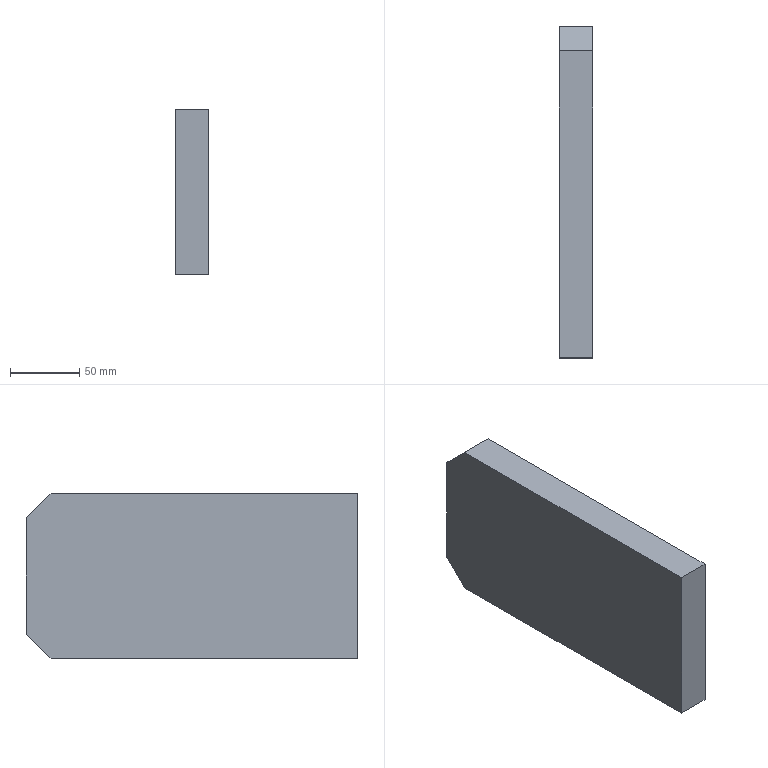Part | NX | 1 solid | 8 faces | box 24 x 240 x 120 mm | volume 683424 mm3 | plane 8
STEP:
#1=CARTESIAN_POINT('',(-235.326,-487.347,2383.086));
#2=VERTEX_POINT('',#1);
#3=CARTESIAN_POINT('',(-235.326,-487.347,2467.086));
#4=VERTEX_POINT('',#3);
#5=CARTESIAN_POINT('',(-235.326,-487.347,2485.086));
#6=DIRECTION('',(0.,0.,1.));
#7=VECTOR('',#6,1.);
#8=LINE('',#5,#7);
#9=EDGE_CURVE('',#2,#4,#8,.T.);
#10=ORIENTED_EDGE('',*,*,#9,.F.);
#11=CARTESIAN_POINT('',(-235.326,-505.347,2365.086));
#12=VERTEX_POINT('',#11);
#13=CARTESIAN_POINT('',(-235.326,-487.347,2383.086));
#14=DIRECTION('',(0.,-0.7071,-0.7071));
#15=VECTOR('',#14,1.);
#16=LINE('',#13,#15);
#17=EDGE_CURVE('',#2,#12,#16,.T.);
#18=ORIENTED_EDGE('',*,*,#17,.T.);
#19=CARTESIAN_POINT('',(-235.326,-727.347,2365.086));
#20=VERTEX_POINT('',#19);
#21=CARTESIAN_POINT('',(-235.326,-487.347,2365.086));
#22=DIRECTION('',(0.,-1.,0.));
#23=VECTOR('',#22,1.);
#24=LINE('',#21,#23);
#25=EDGE_CURVE('',#12,#20,#24,.T.);
#26=ORIENTED_EDGE('',*,*,#25,.T.);
#27=CARTESIAN_POINT('',(-235.326,-727.347,2485.086));
#28=VERTEX_POINT('',#27);
#29=CARTESIAN_POINT('',(-235.326,-727.347,2485.086));
#30=DIRECTION('',(0.,0.,1.));
#31=VECTOR('',#30,1.);
#32=LINE('',#29,#31);
#33=EDGE_CURVE('',#20,#28,#32,.T.);
#34=ORIENTED_EDGE('',*,*,#33,.T.);
#35=CARTESIAN_POINT('',(-235.326,-505.347,2485.086));
#36=VERTEX_POINT('',#35);
#37=CARTESIAN_POINT('',(-235.326,-487.347,2485.086));
#38=DIRECTION('',(0.,-1.,0.));
#39=VECTOR('',#38,1.);
#40=LINE('',#37,#39);
#41=EDGE_CURVE('',#36,#28,#40,.T.);
#42=ORIENTED_EDGE('',*,*,#41,.F.);
#43=CARTESIAN_POINT('',(-235.326,-487.347,2467.086));
#44=DIRECTION('',(0.,0.7071,-0.7071));
#45=VECTOR('',#44,1.);
#46=LINE('',#43,#45);
#47=EDGE_CURVE('',#36,#4,#46,.T.);
#48=ORIENTED_EDGE('',*,*,#47,.T.);
#49=EDGE_LOOP('',(#10,#18,#26,#34,#42,#48));
#50=FACE_OUTER_BOUND('',#49,.T.);
#51=CARTESIAN_POINT('',(-235.326,-487.347,2485.086));
#52=DIRECTION('',(1.,0.,0.));
#53=DIRECTION('',(0.,0.,-1.));
#54=AXIS2_PLACEMENT_3D('',#51,#52,#53);
#55=PLANE('',#54);
#56=ADVANCED_FACE('',(#50),#55,.F.);
#57=CARTESIAN_POINT('',(-211.326,-505.347,2485.086));
#58=VERTEX_POINT('',#57);
#59=CARTESIAN_POINT('',(-211.326,-727.347,2485.086));
#60=VERTEX_POINT('',#59);
#61=CARTESIAN_POINT('',(-211.326,-487.347,2485.086));
#62=DIRECTION('',(0.,-1.,0.));
#63=VECTOR('',#62,1.);
#64=LINE('',#61,#63);
#65=EDGE_CURVE('',#58,#60,#64,.T.);
#66=ORIENTED_EDGE('',*,*,#65,.F.);
#67=CARTESIAN_POINT('',(-235.326,-505.347,2485.086));
#68=DIRECTION('',(-1.,0.,0.));
#69=VECTOR('',#68,1.);
#70=LINE('',#67,#69);
#71=EDGE_CURVE('',#58,#36,#70,.T.);
#72=ORIENTED_EDGE('',*,*,#71,.T.);
#73=ORIENTED_EDGE('',*,*,#41,.T.);
#74=CARTESIAN_POINT('',(-235.326,-727.347,2485.086));
#75=DIRECTION('',(1.,0.,0.));
#76=VECTOR('',#75,1.);
#77=LINE('',#74,#76);
#78=EDGE_CURVE('',#28,#60,#77,.T.);
#79=ORIENTED_EDGE('',*,*,#78,.T.);
#80=EDGE_LOOP('',(#66,#72,#73,#79));
#81=FACE_OUTER_BOUND('',#80,.T.);
#82=CARTESIAN_POINT('',(-235.326,-487.347,2485.086));
#83=DIRECTION('',(0.,0.,-1.));
#84=DIRECTION('',(-1.,0.,0.));
#85=AXIS2_PLACEMENT_3D('',#82,#83,#84);
#86=PLANE('',#85);
#87=ADVANCED_FACE('',(#81),#86,.F.);
#88=CARTESIAN_POINT('',(-211.326,-505.347,2365.086));
#89=VERTEX_POINT('',#88);
#90=CARTESIAN_POINT('',(-211.326,-727.347,2365.086));
#91=VERTEX_POINT('',#90);
#92=CARTESIAN_POINT('',(-211.326,-487.347,2365.086));
#93=DIRECTION('',(0.,-1.,0.));
#94=VECTOR('',#93,1.);
#95=LINE('',#92,#94);
#96=EDGE_CURVE('',#89,#91,#95,.T.);
#97=ORIENTED_EDGE('',*,*,#96,.F.);
#98=CARTESIAN_POINT('',(-211.326,-487.347,2383.086));
#99=VERTEX_POINT('',#98);
#100=CARTESIAN_POINT('',(-211.326,-487.347,2383.086));
#101=DIRECTION('',(0.,0.7071,0.7071));
#102=VECTOR('',#101,1.);
#103=LINE('',#100,#102);
#104=EDGE_CURVE('',#89,#99,#103,.T.);
#105=ORIENTED_EDGE('',*,*,#104,.T.);
#106=CARTESIAN_POINT('',(-211.326,-487.347,2467.086));
#107=VERTEX_POINT('',#106);
#108=CARTESIAN_POINT('',(-211.326,-487.347,2485.086));
#109=DIRECTION('',(0.,0.,-1.));
#110=VECTOR('',#109,1.);
#111=LINE('',#108,#110);
#112=EDGE_CURVE('',#107,#99,#111,.T.);
#113=ORIENTED_EDGE('',*,*,#112,.F.);
#114=CARTESIAN_POINT('',(-211.326,-487.347,2467.086));
#115=DIRECTION('',(0.,-0.7071,0.7071));
#116=VECTOR('',#115,1.);
#117=LINE('',#114,#116);
#118=EDGE_CURVE('',#107,#58,#117,.T.);
#119=ORIENTED_EDGE('',*,*,#118,.T.);
#120=ORIENTED_EDGE('',*,*,#65,.T.);
#121=CARTESIAN_POINT('',(-211.326,-727.347,2485.086));
#122=DIRECTION('',(0.,0.,-1.));
#123=VECTOR('',#122,1.);
#124=LINE('',#121,#123);
#125=EDGE_CURVE('',#60,#91,#124,.T.);
#126=ORIENTED_EDGE('',*,*,#125,.T.);
#127=EDGE_LOOP('',(#97,#105,#113,#119,#120,#126));
#128=FACE_OUTER_BOUND('',#127,.T.);
#129=CARTESIAN_POINT('',(-211.326,-487.347,2485.086));
#130=DIRECTION('',(-1.,0.,0.));
#131=DIRECTION('',(0.,0.,1.));
#132=AXIS2_PLACEMENT_3D('',#129,#130,#131);
#133=PLANE('',#132);
#134=ADVANCED_FACE('',(#128),#133,.F.);
#135=ORIENTED_EDGE('',*,*,#25,.F.);
#136=CARTESIAN_POINT('',(-235.326,-505.347,2365.086));
#137=DIRECTION('',(1.,0.,0.));
#138=VECTOR('',#137,1.);
#139=LINE('',#136,#138);
#140=EDGE_CURVE('',#12,#89,#139,.T.);
#141=ORIENTED_EDGE('',*,*,#140,.T.);
#142=ORIENTED_EDGE('',*,*,#96,.T.);
#143=CARTESIAN_POINT('',(-235.326,-727.347,2365.086));
#144=DIRECTION('',(-1.,0.,0.));
#145=VECTOR('',#144,1.);
#146=LINE('',#143,#145);
#147=EDGE_CURVE('',#91,#20,#146,.T.);
#148=ORIENTED_EDGE('',*,*,#147,.T.);
#149=EDGE_LOOP('',(#135,#141,#142,#148));
#150=FACE_OUTER_BOUND('',#149,.T.);
#151=CARTESIAN_POINT('',(-235.326,-487.347,2365.086));
#152=DIRECTION('',(0.,0.,1.));
#153=DIRECTION('',(1.,0.,0.));
#154=AXIS2_PLACEMENT_3D('',#151,#152,#153);
#155=PLANE('',#154);
#156=ADVANCED_FACE('',(#150),#155,.F.);
#157=ORIENTED_EDGE('',*,*,#112,.T.);
#158=CARTESIAN_POINT('',(-235.326,-487.347,2383.086));
#159=DIRECTION('',(-1.,0.,0.));
#160=VECTOR('',#159,1.);
#161=LINE('',#158,#160);
#162=EDGE_CURVE('',#99,#2,#161,.T.);
#163=ORIENTED_EDGE('',*,*,#162,.T.);
#164=ORIENTED_EDGE('',*,*,#9,.T.);
#165=CARTESIAN_POINT('',(-235.326,-487.347,2467.086));
#166=DIRECTION('',(1.,0.,0.));
#167=VECTOR('',#166,1.);
#168=LINE('',#165,#167);
#169=EDGE_CURVE('',#4,#107,#168,.T.);
#170=ORIENTED_EDGE('',*,*,#169,.T.);
#171=EDGE_LOOP('',(#157,#163,#164,#170));
#172=FACE_OUTER_BOUND('',#171,.T.);
#173=CARTESIAN_POINT('',(-235.326,-487.347,2365.086));
#174=DIRECTION('',(0.,-1.,0.));
#175=DIRECTION('',(0.,0.,-1.));
#176=AXIS2_PLACEMENT_3D('',#173,#174,#175);
#177=PLANE('',#176);
#178=ADVANCED_FACE('',(#172),#177,.F.);
#179=ORIENTED_EDGE('',*,*,#33,.F.);
#180=ORIENTED_EDGE('',*,*,#147,.F.);
#181=ORIENTED_EDGE('',*,*,#125,.F.);
#182=ORIENTED_EDGE('',*,*,#78,.F.);
#183=EDGE_LOOP('',(#179,#180,#181,#182));
#184=FACE_OUTER_BOUND('',#183,.T.);
#185=CARTESIAN_POINT('',(-235.326,-727.347,2365.086));
#186=DIRECTION('',(0.,-1.,0.));
#187=DIRECTION('',(0.,0.,-1.));
#188=AXIS2_PLACEMENT_3D('',#185,#186,#187);
#189=PLANE('',#188);
#190=ADVANCED_FACE('',(#184),#189,.T.);
#191=ORIENTED_EDGE('',*,*,#104,.F.);
#192=ORIENTED_EDGE('',*,*,#140,.F.);
#193=ORIENTED_EDGE('',*,*,#17,.F.);
#194=ORIENTED_EDGE('',*,*,#162,.F.);
#195=EDGE_LOOP('',(#191,#192,#193,#194));
#196=FACE_OUTER_BOUND('',#195,.T.);
#197=CARTESIAN_POINT('',(-235.326,-487.347,2383.086));
#198=DIRECTION('',(0.,-0.7071,0.7071));
#199=DIRECTION('',(0.,-0.7071,-0.7071));
#200=AXIS2_PLACEMENT_3D('',#197,#198,#199);
#201=PLANE('',#200);
#202=ADVANCED_FACE('',(#196),#201,.F.);
#203=ORIENTED_EDGE('',*,*,#47,.F.);
#204=ORIENTED_EDGE('',*,*,#71,.F.);
#205=ORIENTED_EDGE('',*,*,#118,.F.);
#206=ORIENTED_EDGE('',*,*,#169,.F.);
#207=EDGE_LOOP('',(#203,#204,#205,#206));
#208=FACE_OUTER_BOUND('',#207,.T.);
#209=CARTESIAN_POINT('',(-235.326,-487.347,2467.086));
#210=DIRECTION('',(0.,-0.7071,-0.7071));
#211=DIRECTION('',(0.,0.7071,-0.7071));
#212=AXIS2_PLACEMENT_3D('',#209,#210,#211);
#213=PLANE('',#212);
#214=ADVANCED_FACE('',(#208),#213,.F.);
#215=CLOSED_SHELL('',(#56,#87,#134,#156,#178,#190,#202,#214));
#216=MANIFOLD_SOLID_BREP('',#215);
#217=(LENGTH_UNIT()NAMED_UNIT(*)SI_UNIT(.MILLI.,.METRE.));
#218=UNCERTAINTY_MEASURE_WITH_UNIT(LENGTH_MEASURE(0.00002),#217,'','');
#219=(NAMED_UNIT(*)PLANE_ANGLE_UNIT()SI_UNIT($,.RADIAN.));
#220=PLANE_ANGLE_MEASURE_WITH_UNIT(PLANE_ANGLE_MEASURE(0.01745),#219);
#221=DIMENSIONAL_EXPONENTS(0.,0.,0.,0.,0.,0.,0.);
#222=(CONVERSION_BASED_UNIT('DEGREE',#220)NAMED_UNIT(#221)PLANE_ANGLE_UNIT());
#223=(NAMED_UNIT(*)SI_UNIT($,.STERADIAN.)SOLID_ANGLE_UNIT());
#224=(GEOMETRIC_REPRESENTATION_CONTEXT(3)GLOBAL_UNCERTAINTY_ASSIGNED_CONTEXT((#218))GLOBAL_UNIT_ASSIGNED_CONTEXT((#217,#222,#223))REPRESENTATION_CONTEXT('',''));
#225=ADVANCED_BREP_SHAPE_REPRESENTATION('',(#216),#224);